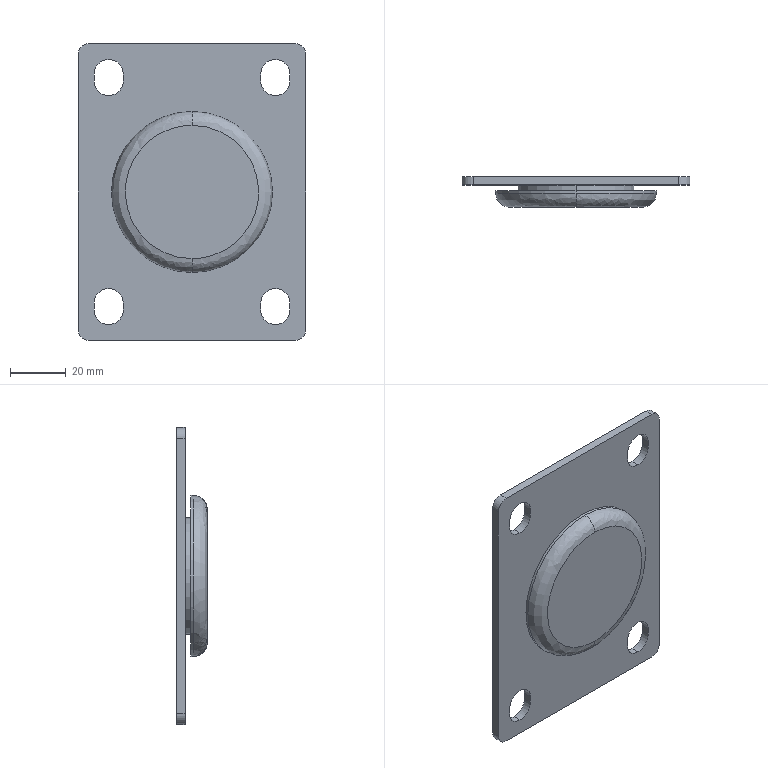Part | SolidWorks | features BaseBody 1 | 1 solid | 47 faces | box 82 x 11 x 107 mm | volume 39892 mm3 | cylinder 26 | plane 19 | spline 2 | commonest cylinder face diameters 10.5 x12 8 x4 25 x2 40 x2 42 x2 58 x2
STEP:
#1=CARTESIAN_POINT('',(0.,55.5,-57.3));
#2=VERTEX_POINT('',#1);
#3=CARTESIAN_POINT('',(0.,55.5,0.7));
#4=VERTEX_POINT('',#3);
#5=CARTESIAN_POINT('',(0.,55.5,-28.3));
#6=DIRECTION('',(0.,1.,0.));
#7=DIRECTION('',(0.,0.,-1.));
#8=AXIS2_PLACEMENT_3D('',#5,#6,#7);
#9=CIRCLE('',#8,29.);
#10=EDGE_CURVE('',#2,#4,#9,.T.);
#11=ORIENTED_EDGE('',*,*,#10,.F.);
#12=CARTESIAN_POINT('',(0.,50.5,-52.3));
#13=VERTEX_POINT('',#12);
#14=CARTESIAN_POINT('',(0.,55.5,-52.3));
#15=DIRECTION('',(-1.,0.,0.));
#16=DIRECTION('',(0.,0.,-1.));
#17=AXIS2_PLACEMENT_3D('',#14,#15,#16);
#18=CIRCLE('',#17,5.);
#19=EDGE_CURVE('',#2,#13,#18,.T.);
#20=ORIENTED_EDGE('',*,*,#19,.T.);
#21=CARTESIAN_POINT('',(0.,50.5,-4.3));
#22=VERTEX_POINT('',#21);
#23=CARTESIAN_POINT('',(0.,50.5,-52.3));
#24=CARTESIAN_POINT('',(-48.,50.5,-52.3));
#25=CARTESIAN_POINT('',(-48.,50.5,-4.3));
#26=CARTESIAN_POINT('',(0.,50.5,-4.3));
#27=(BOUNDED_CURVE()B_SPLINE_CURVE(3,(#23,#24,#25,#26),.UNSPECIFIED.,.F.,.F.)B_SPLINE_CURVE_WITH_KNOTS((4,4),(0.5,1.),.UNSPECIFIED.)CURVE()GEOMETRIC_REPRESENTATION_ITEM()RATIONAL_B_SPLINE_CURVE((1.,0.3333,0.3333,1.))REPRESENTATION_ITEM(''));
#28=EDGE_CURVE('',#13,#22,#27,.T.);
#29=ORIENTED_EDGE('',*,*,#28,.T.);
#30=CARTESIAN_POINT('',(0.,55.5,-4.3));
#31=DIRECTION('',(1.,0.,0.));
#32=DIRECTION('',(0.,0.,1.));
#33=AXIS2_PLACEMENT_3D('',#30,#31,#32);
#34=CIRCLE('',#33,5.);
#35=EDGE_CURVE('',#4,#22,#34,.T.);
#36=ORIENTED_EDGE('',*,*,#35,.F.);
#37=EDGE_LOOP('',(#11,#20,#29,#36));
#38=FACE_OUTER_BOUND('',#37,.T.);
#39=CARTESIAN_POINT('',(0.,55.5,-57.3));
#40=CARTESIAN_POINT('',(-58.,55.5,-57.3));
#41=CARTESIAN_POINT('',(-58.,55.5,0.7));
#42=CARTESIAN_POINT('',(0.,55.5,0.7));
#43=CARTESIAN_POINT('',(0.,52.571,-57.3));
#44=CARTESIAN_POINT('',(-58.,52.571,-57.3));
#45=CARTESIAN_POINT('',(-58.,52.571,0.7));
#46=CARTESIAN_POINT('',(0.,52.571,0.7));
#47=CARTESIAN_POINT('',(0.,50.5,-55.229));
#48=CARTESIAN_POINT('',(-53.858,50.5,-55.229));
#49=CARTESIAN_POINT('',(-53.858,50.5,-1.371));
#50=CARTESIAN_POINT('',(0.,50.5,-1.371));
#51=CARTESIAN_POINT('',(0.,50.5,-52.3));
#52=CARTESIAN_POINT('',(-48.,50.5,-52.3));
#53=CARTESIAN_POINT('',(-48.,50.5,-4.3));
#54=CARTESIAN_POINT('',(0.,50.5,-4.3));
#55=(BOUNDED_SURFACE()B_SPLINE_SURFACE(3,3,((#39,#40,#41,#42),(#43,#44,#45,#46),(#47,#48,#49,#50),(#51,#52,#53,#54)),.UNSPECIFIED.,.F.,.F.,.F.)B_SPLINE_SURFACE_WITH_KNOTS((4,4),(4,4),(0.,1.),(0.,1.),.UNSPECIFIED.)GEOMETRIC_REPRESENTATION_ITEM()RATIONAL_B_SPLINE_SURFACE(((1.,0.3333,0.3333,1.),(0.8047,0.2682,0.2682,0.8047),(0.8047,0.2682,0.2682,0.8047),(1.,0.3333,0.3333,1.)))REPRESENTATION_ITEM('')SURFACE());
#56=ADVANCED_FACE('',(#38),#55,.T.);
#57=CARTESIAN_POINT('',(30.,61.5,6.45));
#58=VERTEX_POINT('',#57);
#59=CARTESIAN_POINT('',(35.25,61.5,11.7));
#60=VERTEX_POINT('',#59);
#61=CARTESIAN_POINT('',(30.,61.5,11.7));
#62=DIRECTION('',(0.,-1.,0.));
#63=DIRECTION('',(0.,0.,-1.));
#64=AXIS2_PLACEMENT_3D('',#61,#62,#63);
#65=CIRCLE('',#64,5.25);
#66=EDGE_CURVE('',#58,#60,#65,.T.);
#67=ORIENTED_EDGE('',*,*,#66,.F.);
#68=CARTESIAN_POINT('',(30.,58.5,6.45));
#69=VERTEX_POINT('',#68);
#70=CARTESIAN_POINT('',(30.,58.5,6.45));
#71=DIRECTION('',(0.,-1.,0.));
#72=VECTOR('',#71,1000.);
#73=LINE('',#70,#72);
#74=EDGE_CURVE('',#58,#69,#73,.T.);
#75=ORIENTED_EDGE('',*,*,#74,.T.);
#76=CARTESIAN_POINT('',(35.25,58.5,11.7));
#77=VERTEX_POINT('',#76);
#78=CARTESIAN_POINT('',(30.,58.5,11.7));
#79=DIRECTION('',(0.,-1.,0.));
#80=DIRECTION('',(0.,0.,-1.));
#81=AXIS2_PLACEMENT_3D('',#78,#79,#80);
#82=CIRCLE('',#81,5.25);
#83=EDGE_CURVE('',#69,#77,#82,.T.);
#84=ORIENTED_EDGE('',*,*,#83,.T.);
#85=CARTESIAN_POINT('',(35.25,58.5,11.7));
#86=DIRECTION('',(0.,-1.,0.));
#87=VECTOR('',#86,1000.);
#88=LINE('',#85,#87);
#89=EDGE_CURVE('',#60,#77,#88,.T.);
#90=ORIENTED_EDGE('',*,*,#89,.F.);
#91=EDGE_LOOP('',(#67,#75,#84,#90));
#92=FACE_OUTER_BOUND('',#91,.T.);
#93=CARTESIAN_POINT('',(30.,58.5,11.7));
#94=DIRECTION('',(0.,-1.,0.));
#95=DIRECTION('',(0.,0.,-1.));
#96=AXIS2_PLACEMENT_3D('',#93,#94,#95);
#97=CYLINDRICAL_SURFACE('',#96,5.25);
#98=ADVANCED_FACE('',(#92),#97,.F.);
#99=CARTESIAN_POINT('',(30.,61.5,-76.05));
#100=VERTEX_POINT('',#99);
#101=CARTESIAN_POINT('',(35.25,61.5,-70.8));
#102=VERTEX_POINT('',#101);
#103=CARTESIAN_POINT('',(30.,61.5,-70.8));
#104=DIRECTION('',(0.,-1.,0.));
#105=DIRECTION('',(0.,0.,-1.));
#106=AXIS2_PLACEMENT_3D('',#103,#104,#105);
#107=CIRCLE('',#106,5.25);
#108=EDGE_CURVE('',#100,#102,#107,.T.);
#109=ORIENTED_EDGE('',*,*,#108,.F.);
#110=CARTESIAN_POINT('',(30.,58.5,-76.05));
#111=VERTEX_POINT('',#110);
#112=CARTESIAN_POINT('',(30.,58.5,-76.05));
#113=DIRECTION('',(0.,-1.,0.));
#114=VECTOR('',#113,1000.);
#115=LINE('',#112,#114);
#116=EDGE_CURVE('',#100,#111,#115,.T.);
#117=ORIENTED_EDGE('',*,*,#116,.T.);
#118=CARTESIAN_POINT('',(35.25,58.5,-70.8));
#119=VERTEX_POINT('',#118);
#120=CARTESIAN_POINT('',(30.,58.5,-70.8));
#121=DIRECTION('',(0.,-1.,0.));
#122=DIRECTION('',(0.,0.,-1.));
#123=AXIS2_PLACEMENT_3D('',#120,#121,#122);
#124=CIRCLE('',#123,5.25);
#125=EDGE_CURVE('',#111,#119,#124,.T.);
#126=ORIENTED_EDGE('',*,*,#125,.T.);
#127=CARTESIAN_POINT('',(35.25,58.5,-70.8));
#128=DIRECTION('',(0.,1.,0.));
#129=VECTOR('',#128,1000.);
#130=LINE('',#127,#129);
#131=EDGE_CURVE('',#119,#102,#130,.T.);
#132=ORIENTED_EDGE('',*,*,#131,.T.);
#133=EDGE_LOOP('',(#109,#117,#126,#132));
#134=FACE_OUTER_BOUND('',#133,.T.);
#135=CARTESIAN_POINT('',(30.,58.5,-70.8));
#136=DIRECTION('',(0.,-1.,0.));
#137=DIRECTION('',(0.,0.,-1.));
#138=AXIS2_PLACEMENT_3D('',#135,#136,#137);
#139=CYLINDRICAL_SURFACE('',#138,5.25);
#140=ADVANCED_FACE('',(#134),#139,.F.);
#141=CARTESIAN_POINT('',(-30.,61.5,6.45));
#142=VERTEX_POINT('',#141);
#143=CARTESIAN_POINT('',(-24.75,61.5,11.7));
#144=VERTEX_POINT('',#143);
#145=CARTESIAN_POINT('',(-30.,61.5,11.7));
#146=DIRECTION('',(0.,-1.,0.));
#147=DIRECTION('',(0.,0.,-1.));
#148=AXIS2_PLACEMENT_3D('',#145,#146,#147);
#149=CIRCLE('',#148,5.25);
#150=EDGE_CURVE('',#142,#144,#149,.T.);
#151=ORIENTED_EDGE('',*,*,#150,.F.);
#152=CARTESIAN_POINT('',(-30.,58.5,6.45));
#153=VERTEX_POINT('',#152);
#154=CARTESIAN_POINT('',(-30.,58.5,6.45));
#155=DIRECTION('',(0.,-1.,0.));
#156=VECTOR('',#155,1000.);
#157=LINE('',#154,#156);
#158=EDGE_CURVE('',#142,#153,#157,.T.);
#159=ORIENTED_EDGE('',*,*,#158,.T.);
#160=CARTESIAN_POINT('',(-24.75,58.5,11.7));
#161=VERTEX_POINT('',#160);
#162=CARTESIAN_POINT('',(-30.,58.5,11.7));
#163=DIRECTION('',(0.,-1.,0.));
#164=DIRECTION('',(0.,0.,-1.));
#165=AXIS2_PLACEMENT_3D('',#162,#163,#164);
#166=CIRCLE('',#165,5.25);
#167=EDGE_CURVE('',#153,#161,#166,.T.);
#168=ORIENTED_EDGE('',*,*,#167,.T.);
#169=CARTESIAN_POINT('',(-24.75,58.5,11.7));
#170=DIRECTION('',(0.,-1.,0.));
#171=VECTOR('',#170,1000.);
#172=LINE('',#169,#171);
#173=EDGE_CURVE('',#144,#161,#172,.T.);
#174=ORIENTED_EDGE('',*,*,#173,.F.);
#175=EDGE_LOOP('',(#151,#159,#168,#174));
#176=FACE_OUTER_BOUND('',#175,.T.);
#177=CARTESIAN_POINT('',(-30.,58.5,11.7));
#178=DIRECTION('',(0.,-1.,0.));
#179=DIRECTION('',(0.,0.,-1.));
#180=AXIS2_PLACEMENT_3D('',#177,#178,#179);
#181=CYLINDRICAL_SURFACE('',#180,5.25);
#182=ADVANCED_FACE('',(#176),#181,.F.);
#183=CARTESIAN_POINT('',(-30.,61.5,-76.05));
#184=VERTEX_POINT('',#183);
#185=CARTESIAN_POINT('',(-24.75,61.5,-70.8));
#186=VERTEX_POINT('',#185);
#187=CARTESIAN_POINT('',(-30.,61.5,-70.8));
#188=DIRECTION('',(0.,-1.,0.));
#189=DIRECTION('',(0.,0.,-1.));
#190=AXIS2_PLACEMENT_3D('',#187,#188,#189);
#191=CIRCLE('',#190,5.25);
#192=EDGE_CURVE('',#184,#186,#191,.T.);
#193=ORIENTED_EDGE('',*,*,#192,.F.);
#194=CARTESIAN_POINT('',(-30.,58.5,-76.05));
#195=VERTEX_POINT('',#194);
#196=CARTESIAN_POINT('',(-30.,58.5,-76.05));
#197=DIRECTION('',(0.,-1.,0.));
#198=VECTOR('',#197,1000.);
#199=LINE('',#196,#198);
#200=EDGE_CURVE('',#184,#195,#199,.T.);
#201=ORIENTED_EDGE('',*,*,#200,.T.);
#202=CARTESIAN_POINT('',(-24.75,58.5,-70.8));
#203=VERTEX_POINT('',#202);
#204=CARTESIAN_POINT('',(-30.,58.5,-70.8));
#205=DIRECTION('',(0.,-1.,0.));
#206=DIRECTION('',(0.,0.,-1.));
#207=AXIS2_PLACEMENT_3D('',#204,#205,#206);
#208=CIRCLE('',#207,5.25);
#209=EDGE_CURVE('',#195,#203,#208,.T.);
#210=ORIENTED_EDGE('',*,*,#209,.T.);
#211=CARTESIAN_POINT('',(-24.75,58.5,-70.8));
#212=DIRECTION('',(0.,1.,0.));
#213=VECTOR('',#212,1000.);
#214=LINE('',#211,#213);
#215=EDGE_CURVE('',#203,#186,#214,.T.);
#216=ORIENTED_EDGE('',*,*,#215,.T.);
#217=EDGE_LOOP('',(#193,#201,#210,#216));
#218=FACE_OUTER_BOUND('',#217,.T.);
#219=CARTESIAN_POINT('',(-30.,58.5,-70.8));
#220=DIRECTION('',(0.,-1.,0.));
#221=DIRECTION('',(0.,0.,-1.));
#222=AXIS2_PLACEMENT_3D('',#219,#220,#221);
#223=CYLINDRICAL_SURFACE('',#222,5.25);
#224=ADVANCED_FACE('',(#218),#223,.F.);
#225=CARTESIAN_POINT('',(0.,58.5,-49.3));
#226=VERTEX_POINT('',#225);
#227=CARTESIAN_POINT('',(0.,58.5,-7.3));
#228=VERTEX_POINT('',#227);
#229=CARTESIAN_POINT('',(0.,58.5,-28.3));
#230=DIRECTION('',(0.,-1.,0.));
#231=DIRECTION('',(0.,0.,-1.));
#232=AXIS2_PLACEMENT_3D('',#229,#230,#231);
#233=CIRCLE('',#232,21.);
#234=EDGE_CURVE('',#226,#228,#233,.T.);
#235=ORIENTED_EDGE('',*,*,#234,.T.);
#236=CARTESIAN_POINT('',(0.,56.5,-7.3));
#237=VERTEX_POINT('',#236);
#238=CARTESIAN_POINT('',(0.,56.5,-7.3));
#239=DIRECTION('',(0.,-1.,0.));
#240=VECTOR('',#239,1000.);
#241=LINE('',#238,#240);
#242=EDGE_CURVE('',#228,#237,#241,.T.);
#243=ORIENTED_EDGE('',*,*,#242,.T.);
#244=CARTESIAN_POINT('',(0.,56.5,-49.3));
#245=VERTEX_POINT('',#244);
#246=CARTESIAN_POINT('',(0.,56.5,-28.3));
#247=DIRECTION('',(0.,1.,0.));
#248=DIRECTION('',(0.,0.,-1.));
#249=AXIS2_PLACEMENT_3D('',#246,#247,#248);
#250=CIRCLE('',#249,21.);
#251=EDGE_CURVE('',#237,#245,#250,.T.);
#252=ORIENTED_EDGE('',*,*,#251,.T.);
#253=CARTESIAN_POINT('',(0.,56.5,-49.3));
#254=DIRECTION('',(0.,-1.,0.));
#255=VECTOR('',#254,1000.);
#256=LINE('',#253,#255);
#257=EDGE_CURVE('',#226,#245,#256,.T.);
#258=ORIENTED_EDGE('',*,*,#257,.F.);
#259=EDGE_LOOP('',(#235,#243,#252,#258));
#260=FACE_OUTER_BOUND('',#259,.T.);
#261=CARTESIAN_POINT('',(0.,56.5,-28.3));
#262=DIRECTION('',(0.,-1.,0.));
#263=DIRECTION('',(0.,0.,-1.));
#264=AXIS2_PLACEMENT_3D('',#261,#262,#263);
#265=CYLINDRICAL_SURFACE('',#264,21.);
#266=ADVANCED_FACE('',(#260),#265,.T.);
#267=CARTESIAN_POINT('',(0.,61.5,1.7));
#268=VERTEX_POINT('',#267);
#269=CARTESIAN_POINT('',(0.,61.5,-58.3));
#270=VERTEX_POINT('',#269);
#271=CARTESIAN_POINT('',(0.,61.5,-28.3));
#272=DIRECTION('',(0.,-1.,0.));
#273=DIRECTION('',(0.,0.,-1.));
#274=AXIS2_PLACEMENT_3D('',#271,#272,#273);
#275=CIRCLE('',#274,30.);
#276=EDGE_CURVE('',#268,#270,#275,.T.);
#277=ORIENTED_EDGE('',*,*,#276,.F.);
#278=CARTESIAN_POINT('',(0.,60.5,1.7));
#279=VERTEX_POINT('',#278);
#280=CARTESIAN_POINT('',(0.,60.5,1.7));
#281=DIRECTION('',(0.,-1.,0.));
#282=VECTOR('',#281,1000.);
#283=LINE('',#280,#282);
#284=EDGE_CURVE('',#268,#279,#283,.T.);
#285=ORIENTED_EDGE('',*,*,#284,.T.);
#286=CARTESIAN_POINT('',(0.,60.5,-58.3));
#287=VERTEX_POINT('',#286);
#288=CARTESIAN_POINT('',(0.,60.5,-28.3));
#289=DIRECTION('',(0.,1.,0.));
#290=DIRECTION('',(0.,0.,-1.));
#291=AXIS2_PLACEMENT_3D('',#288,#289,#290);
#292=CIRCLE('',#291,30.);
#293=EDGE_CURVE('',#287,#279,#292,.T.);
#294=ORIENTED_EDGE('',*,*,#293,.F.);
#295=CARTESIAN_POINT('',(0.,60.5,-58.3));
#296=DIRECTION('',(0.,-1.,0.));
#297=VECTOR('',#296,1000.);
#298=LINE('',#295,#297);
#299=EDGE_CURVE('',#270,#287,#298,.T.);
#300=ORIENTED_EDGE('',*,*,#299,.F.);
#301=EDGE_LOOP('',(#277,#285,#294,#300));
#302=FACE_OUTER_BOUND('',#301,.T.);
#303=CARTESIAN_POINT('',(0.,60.5,-28.3));
#304=DIRECTION('',(0.,-1.,0.));
#305=DIRECTION('',(0.,0.,-1.));
#306=AXIS2_PLACEMENT_3D('',#303,#304,#305);
#307=CYLINDRICAL_SURFACE('',#306,30.);
#308=ADVANCED_FACE('',(#302),#307,.F.);
#309=CARTESIAN_POINT('',(0.,56.5,-57.3));
#310=VERTEX_POINT('',#309);
#311=CARTESIAN_POINT('',(0.,56.5,0.7));
#312=VERTEX_POINT('',#311);
#313=CARTESIAN_POINT('',(0.,56.5,-28.3));
#314=DIRECTION('',(0.,-1.,0.));
#315=DIRECTION('',(0.,0.,-1.));
#316=AXIS2_PLACEMENT_3D('',#313,#314,#315);
#317=CIRCLE('',#316,29.);
#318=EDGE_CURVE('',#310,#312,#317,.T.);
#319=ORIENTED_EDGE('',*,*,#318,.T.);
#320=CARTESIAN_POINT('',(0.,56.5,0.7));
#321=DIRECTION('',(0.,-1.,0.));
#322=VECTOR('',#321,1000.);
#323=LINE('',#320,#322);
#324=EDGE_CURVE('',#312,#4,#323,.T.);
#325=ORIENTED_EDGE('',*,*,#324,.T.);
#326=CARTESIAN_POINT('',(0.,55.5,-28.3));
#327=DIRECTION('',(0.,1.,0.));
#328=DIRECTION('',(0.,0.,-1.));
#329=AXIS2_PLACEMENT_3D('',#326,#327,#328);
#330=CIRCLE('',#329,29.);
#331=EDGE_CURVE('',#4,#2,#330,.T.);
#332=ORIENTED_EDGE('',*,*,#331,.T.);
#333=CARTESIAN_POINT('',(0.,56.5,-57.3));
#334=DIRECTION('',(0.,-1.,0.));
#335=VECTOR('',#334,1000.);
#336=LINE('',#333,#335);
#337=EDGE_CURVE('',#310,#2,#336,.T.);
#338=ORIENTED_EDGE('',*,*,#337,.F.);
#339=EDGE_LOOP('',(#319,#325,#332,#338));
#340=FACE_OUTER_BOUND('',#339,.T.);
#341=CARTESIAN_POINT('',(0.,56.5,-28.3));
#342=DIRECTION('',(0.,-1.,0.));
#343=DIRECTION('',(0.,0.,-1.));
#344=AXIS2_PLACEMENT_3D('',#341,#342,#343);
#345=CYLINDRICAL_SURFACE('',#344,29.);
#346=ADVANCED_FACE('',(#340),#345,.T.);
#347=CARTESIAN_POINT('',(0.,60.5,-8.3));
#348=VERTEX_POINT('',#347);
#349=CARTESIAN_POINT('',(0.,60.5,-48.3));
#350=VERTEX_POINT('',#349);
#351=CARTESIAN_POINT('',(0.,60.5,-28.3));
#352=DIRECTION('',(0.,-1.,0.));
#353=DIRECTION('',(0.,0.,-1.));
#354=AXIS2_PLACEMENT_3D('',#351,#352,#353);
#355=CIRCLE('',#354,20.);
#356=EDGE_CURVE('',#348,#350,#355,.T.);
#357=ORIENTED_EDGE('',*,*,#356,.F.);
#358=CARTESIAN_POINT('',(0.,60.,-8.3));
#359=VERTEX_POINT('',#358);
#360=CARTESIAN_POINT('',(0.,60.,-8.3));
#361=DIRECTION('',(0.,-1.,0.));
#362=VECTOR('',#361,1000.);
#363=LINE('',#360,#362);
#364=EDGE_CURVE('',#348,#359,#363,.T.);
#365=ORIENTED_EDGE('',*,*,#364,.T.);
#366=CARTESIAN_POINT('',(0.,60.,-48.3));
#367=VERTEX_POINT('',#366);
#368=CARTESIAN_POINT('',(0.,60.,-28.3));
#369=DIRECTION('',(0.,1.,0.));
#370=DIRECTION('',(0.,0.,-1.));
#371=AXIS2_PLACEMENT_3D('',#368,#369,#370);
#372=CIRCLE('',#371,20.);
#373=EDGE_CURVE('',#367,#359,#372,.T.);
#374=ORIENTED_EDGE('',*,*,#373,.F.);
#375=CARTESIAN_POINT('',(0.,60.,-48.3));
#376=DIRECTION('',(0.,-1.,0.));
#377=VECTOR('',#376,1000.);
#378=LINE('',#375,#377);
#379=EDGE_CURVE('',#350,#367,#378,.T.);
#380=ORIENTED_EDGE('',*,*,#379,.F.);
#381=EDGE_LOOP('',(#357,#365,#374,#380));
#382=FACE_OUTER_BOUND('',#381,.T.);
#383=CARTESIAN_POINT('',(0.,60.,-28.3));
#384=DIRECTION('',(0.,-1.,0.));
#385=DIRECTION('',(0.,0.,-1.));
#386=AXIS2_PLACEMENT_3D('',#383,#384,#385);
#387=CYLINDRICAL_SURFACE('',#386,20.);
#388=ADVANCED_FACE('',(#382),#387,.F.);
#389=CARTESIAN_POINT('',(0.,61.5,-40.8));
#390=VERTEX_POINT('',#389);
#391=CARTESIAN_POINT('',(0.,61.5,-15.8));
#392=VERTEX_POINT('',#391);
#393=CARTESIAN_POINT('',(0.,61.5,-28.3));
#394=DIRECTION('',(0.,-1.,0.));
#395=DIRECTION('',(0.,0.,-1.));
#396=AXIS2_PLACEMENT_3D('',#393,#394,#395);
#397=CIRCLE('',#396,12.5);
#398=EDGE_CURVE('',#390,#392,#397,.T.);
#399=ORIENTED_EDGE('',*,*,#398,.T.);
#400=CARTESIAN_POINT('',(0.,60.,-15.8));
#401=VERTEX_POINT('',#400);
#402=CARTESIAN_POINT('',(0.,59.,-15.8));
#403=DIRECTION('',(0.,-1.,0.));
#404=VECTOR('',#403,1000.);
#405=LINE('',#402,#404);
#406=EDGE_CURVE('',#392,#401,#405,.T.);
#407=ORIENTED_EDGE('',*,*,#406,.T.);
#408=CARTESIAN_POINT('',(0.,60.,-40.8));
#409=VERTEX_POINT('',#408);
#410=CARTESIAN_POINT('',(0.,60.,-28.3));
#411=DIRECTION('',(0.,-1.,0.));
#412=DIRECTION('',(0.,0.,-1.));
#413=AXIS2_PLACEMENT_3D('',#410,#411,#412);
#414=CIRCLE('',#413,12.5);
#415=EDGE_CURVE('',#409,#401,#414,.T.);
#416=ORIENTED_EDGE('',*,*,#415,.F.);
#417=CARTESIAN_POINT('',(0.,59.,-40.8));
#418=DIRECTION('',(0.,-1.,0.));
#419=VECTOR('',#418,1000.);
#420=LINE('',#417,#419);
#421=EDGE_CURVE('',#390,#409,#420,.T.);
#422=ORIENTED_EDGE('',*,*,#421,.F.);
#423=EDGE_LOOP('',(#399,#407,#416,#422));
#424=FACE_OUTER_BOUND('',#423,.T.);
#425=CARTESIAN_POINT('',(0.,59.,-28.3));
#426=DIRECTION('',(0.,-1.,0.));
#427=DIRECTION('',(0.,0.,-1.));
#428=AXIS2_PLACEMENT_3D('',#425,#426,#427);
#429=CYLINDRICAL_SURFACE('',#428,12.5);
#430=ADVANCED_FACE('',(#424),#429,.T.);
#431=CARTESIAN_POINT('',(37.,58.5,-81.8));
#432=VERTEX_POINT('',#431);
#433=CARTESIAN_POINT('',(-37.,58.5,-81.8));
#434=VERTEX_POINT('',#433);
#435=CARTESIAN_POINT('',(-37.,58.5,-81.8));
#436=DIRECTION('',(-1.,0.,0.));
#437=VECTOR('',#436,1000.);
#438=LINE('',#435,#437);
#439=EDGE_CURVE('',#432,#434,#438,.T.);
#440=ORIENTED_EDGE('',*,*,#439,.F.);
#441=CARTESIAN_POINT('',(41.,58.5,-77.8));
#442=VERTEX_POINT('',#441);
#443=CARTESIAN_POINT('',(37.,58.5,-77.8));
#444=DIRECTION('',(0.,1.,0.));
#445=DIRECTION('',(0.,0.,-1.));
#446=AXIS2_PLACEMENT_3D('',#443,#444,#445);
#447=CIRCLE('',#446,4.);
#448=EDGE_CURVE('',#442,#432,#447,.T.);
#449=ORIENTED_EDGE('',*,*,#448,.F.);
#450=CARTESIAN_POINT('',(41.,58.5,21.2));
#451=VERTEX_POINT('',#450);
#452=CARTESIAN_POINT('',(41.,58.5,-77.8));
#453=DIRECTION('',(0.,0.,-1.));
#454=VECTOR('',#453,1000.);
#455=LINE('',#452,#454);
#456=EDGE_CURVE('',#451,#442,#455,.T.);
#457=ORIENTED_EDGE('',*,*,#456,.F.);
#458=CARTESIAN_POINT('',(37.,58.5,25.2));
#459=VERTEX_POINT('',#458);
#460=CARTESIAN_POINT('',(37.,58.5,21.2));
#461=DIRECTION('',(0.,1.,0.));
#462=DIRECTION('',(0.,0.,-1.));
#463=AXIS2_PLACEMENT_3D('',#460,#461,#462);
#464=CIRCLE('',#463,4.);
#465=EDGE_CURVE('',#459,#451,#464,.T.);
#466=ORIENTED_EDGE('',*,*,#465,.F.);
#467=CARTESIAN_POINT('',(-37.,58.5,25.2));
#468=VERTEX_POINT('',#467);
#469=CARTESIAN_POINT('',(-37.,58.5,25.2));
#470=DIRECTION('',(1.,0.,0.));
#471=VECTOR('',#470,1000.);
#472=LINE('',#469,#471);
#473=EDGE_CURVE('',#468,#459,#472,.T.);
#474=ORIENTED_EDGE('',*,*,#473,.F.);
#475=CARTESIAN_POINT('',(-41.,58.5,21.2));
#476=VERTEX_POINT('',#475);
#477=CARTESIAN_POINT('',(-37.,58.5,21.2));
#478=DIRECTION('',(0.,1.,0.));
#479=DIRECTION('',(0.,0.,-1.));
#480=AXIS2_PLACEMENT_3D('',#477,#478,#479);
#481=CIRCLE('',#480,4.);
#482=EDGE_CURVE('',#476,#468,#481,.T.);
#483=ORIENTED_EDGE('',*,*,#482,.F.);
#484=CARTESIAN_POINT('',(-41.,58.5,-77.8));
#485=VERTEX_POINT('',#484);
#486=CARTESIAN_POINT('',(-41.,58.5,-77.8));
#487=DIRECTION('',(0.,0.,1.));
#488=VECTOR('',#487,1000.);
#489=LINE('',#486,#488);
#490=EDGE_CURVE('',#485,#476,#489,.T.);
#491=ORIENTED_EDGE('',*,*,#490,.F.);
#492=CARTESIAN_POINT('',(-37.,58.5,-77.8));
#493=DIRECTION('',(0.,1.,0.));
#494=DIRECTION('',(0.,0.,-1.));
#495=AXIS2_PLACEMENT_3D('',#492,#493,#494);
#496=CIRCLE('',#495,4.);
#497=EDGE_CURVE('',#434,#485,#496,.T.);
#498=ORIENTED_EDGE('',*,*,#497,.F.);
#499=EDGE_LOOP('',(#440,#449,#457,#466,#474,#483,#491,#498));
#500=FACE_OUTER_BOUND('',#499,.T.);
#501=CARTESIAN_POINT('',(24.75,58.5,14.2));
#502=VERTEX_POINT('',#501);
#503=CARTESIAN_POINT('',(24.75,58.5,11.7));
#504=VERTEX_POINT('',#503);
#505=CARTESIAN_POINT('',(24.75,58.5,-77.8));
#506=DIRECTION('',(0.,0.,-1.));
#507=VECTOR('',#506,1000.);
#508=LINE('',#505,#507);
#509=EDGE_CURVE('',#502,#504,#508,.T.);
#510=ORIENTED_EDGE('',*,*,#509,.F.);
#511=CARTESIAN_POINT('',(35.25,58.5,14.2));
#512=VERTEX_POINT('',#511);
#513=CARTESIAN_POINT('',(30.,58.5,14.2));
#514=DIRECTION('',(0.,-1.,0.));
#515=DIRECTION('',(0.,0.,-1.));
#516=AXIS2_PLACEMENT_3D('',#513,#514,#515);
#517=CIRCLE('',#516,5.25);
#518=EDGE_CURVE('',#512,#502,#517,.T.);
#519=ORIENTED_EDGE('',*,*,#518,.F.);
#520=CARTESIAN_POINT('',(35.25,58.5,-77.8));
#521=DIRECTION('',(0.,0.,1.));
#522=VECTOR('',#521,1000.);
#523=LINE('',#520,#522);
#524=EDGE_CURVE('',#77,#512,#523,.T.);
#525=ORIENTED_EDGE('',*,*,#524,.F.);
#526=ORIENTED_EDGE('',*,*,#83,.F.);
#527=CARTESIAN_POINT('',(30.,58.5,11.7));
#528=DIRECTION('',(0.,-1.,0.));
#529=DIRECTION('',(0.,0.,-1.));
#530=AXIS2_PLACEMENT_3D('',#527,#528,#529);
#531=CIRCLE('',#530,5.25);
#532=EDGE_CURVE('',#504,#69,#531,.T.);
#533=ORIENTED_EDGE('',*,*,#532,.F.);
#534=EDGE_LOOP('',(#510,#519,#525,#526,#533));
#535=FACE_BOUND('',#534,.T.);
#536=CARTESIAN_POINT('',(35.25,58.5,-68.3));
#537=VERTEX_POINT('',#536);
#538=CARTESIAN_POINT('',(24.75,58.5,-68.3));
#539=VERTEX_POINT('',#538);
#540=CARTESIAN_POINT('',(30.,58.5,-68.3));
#541=DIRECTION('',(0.,-1.,0.));
#542=DIRECTION('',(0.,0.,-1.));
#543=AXIS2_PLACEMENT_3D('',#540,#541,#542);
#544=CIRCLE('',#543,5.25);
#545=EDGE_CURVE('',#537,#539,#544,.T.);
#546=ORIENTED_EDGE('',*,*,#545,.F.);
#547=CARTESIAN_POINT('',(35.25,58.5,-77.8));
#548=DIRECTION('',(0.,0.,1.));
#549=VECTOR('',#548,1000.);
#550=LINE('',#547,#549);
#551=EDGE_CURVE('',#119,#537,#550,.T.);
#552=ORIENTED_EDGE('',*,*,#551,.F.);
#553=ORIENTED_EDGE('',*,*,#125,.F.);
#554=CARTESIAN_POINT('',(24.75,58.5,-70.8));
#555=VERTEX_POINT('',#554);
#556=CARTESIAN_POINT('',(30.,58.5,-70.8));
#557=DIRECTION('',(0.,-1.,0.));
#558=DIRECTION('',(0.,0.,-1.));
#559=AXIS2_PLACEMENT_3D('',#556,#557,#558);
#560=CIRCLE('',#559,5.25);
#561=EDGE_CURVE('',#555,#111,#560,.T.);
#562=ORIENTED_EDGE('',*,*,#561,.F.);
#563=CARTESIAN_POINT('',(24.75,58.5,-77.8));
#564=DIRECTION('',(0.,0.,-1.));
#565=VECTOR('',#564,1000.);
#566=LINE('',#563,#565);
#567=EDGE_CURVE('',#539,#555,#566,.T.);
#568=ORIENTED_EDGE('',*,*,#567,.F.);
#569=EDGE_LOOP('',(#546,#552,#553,#562,#568));
#570=FACE_BOUND('',#569,.T.);
#571=CARTESIAN_POINT('',(-35.25,58.5,14.2));
#572=VERTEX_POINT('',#571);
#573=CARTESIAN_POINT('',(-35.25,58.5,11.7));
#574=VERTEX_POINT('',#573);
#575=CARTESIAN_POINT('',(-35.25,58.5,-77.8));
#576=DIRECTION('',(0.,0.,-1.));
#577=VECTOR('',#576,1000.);
#578=LINE('',#575,#577);
#579=EDGE_CURVE('',#572,#574,#578,.T.);
#580=ORIENTED_EDGE('',*,*,#579,.F.);
#581=CARTESIAN_POINT('',(-24.75,58.5,14.2));
#582=VERTEX_POINT('',#581);
#583=CARTESIAN_POINT('',(-30.,58.5,14.2));
#584=DIRECTION('',(0.,-1.,0.));
#585=DIRECTION('',(0.,0.,-1.));
#586=AXIS2_PLACEMENT_3D('',#583,#584,#585);
#587=CIRCLE('',#586,5.25);
#588=EDGE_CURVE('',#582,#572,#587,.T.);
#589=ORIENTED_EDGE('',*,*,#588,.F.);
#590=CARTESIAN_POINT('',(-24.75,58.5,-77.8));
#591=DIRECTION('',(0.,0.,1.));
#592=VECTOR('',#591,1000.);
#593=LINE('',#590,#592);
#594=EDGE_CURVE('',#161,#582,#593,.T.);
#595=ORIENTED_EDGE('',*,*,#594,.F.);
#596=ORIENTED_EDGE('',*,*,#167,.F.);
#597=CARTESIAN_POINT('',(-30.,58.5,11.7));
#598=DIRECTION('',(0.,-1.,0.));
#599=DIRECTION('',(0.,0.,-1.));
#600=AXIS2_PLACEMENT_3D('',#597,#598,#599);
#601=CIRCLE('',#600,5.25);
#602=EDGE_CURVE('',#574,#153,#601,.T.);
#603=ORIENTED_EDGE('',*,*,#602,.F.);
#604=EDGE_LOOP('',(#580,#589,#595,#596,#603));
#605=FACE_BOUND('',#604,.T.);
#606=CARTESIAN_POINT('',(-24.75,58.5,-68.3));
#607=VERTEX_POINT('',#606);
#608=CARTESIAN_POINT('',(-35.25,58.5,-68.3));
#609=VERTEX_POINT('',#608);
#610=CARTESIAN_POINT('',(-30.,58.5,-68.3));
#611=DIRECTION('',(0.,-1.,0.));
#612=DIRECTION('',(0.,0.,-1.));
#613=AXIS2_PLACEMENT_3D('',#610,#611,#612);
#614=CIRCLE('',#613,5.25);
#615=EDGE_CURVE('',#607,#609,#614,.T.);
#616=ORIENTED_EDGE('',*,*,#615,.F.);
#617=CARTESIAN_POINT('',(-24.75,58.5,-77.8));
#618=DIRECTION('',(0.,0.,1.));
#619=VECTOR('',#618,1000.);
#620=LINE('',#617,#619);
#621=EDGE_CURVE('',#203,#607,#620,.T.);
#622=ORIENTED_EDGE('',*,*,#621,.F.);
#623=ORIENTED_EDGE('',*,*,#209,.F.);
#624=CARTESIAN_POINT('',(-35.25,58.5,-70.8));
#625=VERTEX_POINT('',#624);
#626=CARTESIAN_POINT('',(-30.,58.5,-70.8));
#627=DIRECTION('',(0.,-1.,0.));
#628=DIRECTION('',(0.,0.,-1.));
#629=AXIS2_PLACEMENT_3D('',#626,#627,#628);
#630=CIRCLE('',#629,5.25);
#631=EDGE_CURVE('',#625,#195,#630,.T.);
#632=ORIENTED_EDGE('',*,*,#631,.F.);
#633=CARTESIAN_POINT('',(-35.25,58.5,-77.8));
#634=DIRECTION('',(0.,0.,-1.));
#635=VECTOR('',#634,1000.);
#636=LINE('',#633,#635);
#637=EDGE_CURVE('',#609,#625,#636,.T.);
#638=ORIENTED_EDGE('',*,*,#637,.F.);
#639=EDGE_LOOP('',(#616,#622,#623,#632,#638));
#640=FACE_BOUND('',#639,.T.);
#641=ORIENTED_EDGE('',*,*,#234,.F.);
#642=CARTESIAN_POINT('',(0.,58.5,-28.3));
#643=DIRECTION('',(0.,-1.,0.));
#644=DIRECTION('',(0.,0.,-1.));
#645=AXIS2_PLACEMENT_3D('',#642,#643,#644);
#646=CIRCLE('',#645,21.);
#647=EDGE_CURVE('',#228,#226,#646,.T.);
#648=ORIENTED_EDGE('',*,*,#647,.F.);
#649=EDGE_LOOP('',(#641,#648));
#650=FACE_BOUND('',#649,.T.);
#651=CARTESIAN_POINT('',(-37.,58.5,-77.8));
#652=DIRECTION('',(0.,1.,0.));
#653=DIRECTION('',(0.,0.,1.));
#654=AXIS2_PLACEMENT_3D('',#651,#652,#653);
#655=PLANE('',#654);
#656=ADVANCED_FACE('',(#500,#535,#570,#605,#640,#650),#655,.F.);
#657=ORIENTED_EDGE('',*,*,#497,.T.);
#658=CARTESIAN_POINT('',(-41.,61.5,-77.8));
#659=VERTEX_POINT('',#658);
#660=CARTESIAN_POINT('',(-41.,58.5,-77.8));
#661=DIRECTION('',(0.,1.,0.));
#662=VECTOR('',#661,1000.);
#663=LINE('',#660,#662);
#664=EDGE_CURVE('',#485,#659,#663,.T.);
#665=ORIENTED_EDGE('',*,*,#664,.T.);
#666=CARTESIAN_POINT('',(-37.,61.5,-81.8));
#667=VERTEX_POINT('',#666);
#668=CARTESIAN_POINT('',(-37.,61.5,-77.8));
#669=DIRECTION('',(0.,-1.,0.));
#670=DIRECTION('',(0.,0.,-1.));
#671=AXIS2_PLACEMENT_3D('',#668,#669,#670);
#672=CIRCLE('',#671,4.);
#673=EDGE_CURVE('',#659,#667,#672,.T.);
#674=ORIENTED_EDGE('',*,*,#673,.T.);
#675=CARTESIAN_POINT('',(-37.,58.5,-81.8));
#676=DIRECTION('',(0.,-1.,0.));
#677=VECTOR('',#676,1000.);
#678=LINE('',#675,#677);
#679=EDGE_CURVE('',#667,#434,#678,.T.);
#680=ORIENTED_EDGE('',*,*,#679,.T.);
#681=EDGE_LOOP('',(#657,#665,#674,#680));
#682=FACE_OUTER_BOUND('',#681,.T.);
#683=CARTESIAN_POINT('',(-37.,58.5,-77.8));
#684=DIRECTION('',(0.,-1.,0.));
#685=DIRECTION('',(0.,0.,-1.));
#686=AXIS2_PLACEMENT_3D('',#683,#684,#685);
#687=CYLINDRICAL_SURFACE('',#686,4.);
#688=ADVANCED_FACE('',(#682),#687,.T.);
#689=ORIENTED_EDGE('',*,*,#439,.T.);
#690=ORIENTED_EDGE('',*,*,#679,.F.);
#691=CARTESIAN_POINT('',(37.,61.5,-81.8));
#692=VERTEX_POINT('',#691);
#693=CARTESIAN_POINT('',(37.,61.5,-81.8));
#694=DIRECTION('',(1.,0.,0.));
#695=VECTOR('',#694,1000.);
#696=LINE('',#693,#695);
#697=EDGE_CURVE('',#667,#692,#696,.T.);
#698=ORIENTED_EDGE('',*,*,#697,.T.);
#699=CARTESIAN_POINT('',(37.,58.5,-81.8));
#700=DIRECTION('',(0.,-1.,0.));
#701=VECTOR('',#700,1000.);
#702=LINE('',#699,#701);
#703=EDGE_CURVE('',#692,#432,#702,.T.);
#704=ORIENTED_EDGE('',*,*,#703,.T.);
#705=EDGE_LOOP('',(#689,#690,#698,#704));
#706=FACE_OUTER_BOUND('',#705,.T.);
#707=CARTESIAN_POINT('',(37.,58.5,-81.8));
#708=DIRECTION('',(0.,0.,-1.));
#709=DIRECTION('',(-1.,0.,0.));
#710=AXIS2_PLACEMENT_3D('',#707,#708,#709);
#711=PLANE('',#710);
#712=ADVANCED_FACE('',(#706),#711,.T.);
#713=ORIENTED_EDGE('',*,*,#448,.T.);
#714=ORIENTED_EDGE('',*,*,#703,.F.);
#715=CARTESIAN_POINT('',(41.,61.5,-77.8));
#716=VERTEX_POINT('',#715);
#717=CARTESIAN_POINT('',(37.,61.5,-77.8));
#718=DIRECTION('',(0.,-1.,0.));
#719=DIRECTION('',(0.,0.,-1.));
#720=AXIS2_PLACEMENT_3D('',#717,#718,#719);
#721=CIRCLE('',#720,4.);
#722=EDGE_CURVE('',#692,#716,#721,.T.);
#723=ORIENTED_EDGE('',*,*,#722,.T.);
#724=CARTESIAN_POINT('',(41.,58.5,-77.8));
#725=DIRECTION('',(0.,-1.,0.));
#726=VECTOR('',#725,1000.);
#727=LINE('',#724,#726);
#728=EDGE_CURVE('',#716,#442,#727,.T.);
#729=ORIENTED_EDGE('',*,*,#728,.T.);
#730=EDGE_LOOP('',(#713,#714,#723,#729));
#731=FACE_OUTER_BOUND('',#730,.T.);
#732=CARTESIAN_POINT('',(37.,58.5,-77.8));
#733=DIRECTION('',(0.,-1.,0.));
#734=DIRECTION('',(0.,0.,-1.));
#735=AXIS2_PLACEMENT_3D('',#732,#733,#734);
#736=CYLINDRICAL_SURFACE('',#735,4.);
#737=ADVANCED_FACE('',(#731),#736,.T.);
#738=ORIENTED_EDGE('',*,*,#456,.T.);
#739=ORIENTED_EDGE('',*,*,#728,.F.);
#740=CARTESIAN_POINT('',(41.,61.5,21.2));
#741=VERTEX_POINT('',#740);
#742=CARTESIAN_POINT('',(41.,61.5,21.2));
#743=DIRECTION('',(0.,0.,1.));
#744=VECTOR('',#743,1000.);
#745=LINE('',#742,#744);
#746=EDGE_CURVE('',#716,#741,#745,.T.);
#747=ORIENTED_EDGE('',*,*,#746,.T.);
#748=CARTESIAN_POINT('',(41.,58.5,21.2));
#749=DIRECTION('',(0.,-1.,0.));
#750=VECTOR('',#749,1000.);
#751=LINE('',#748,#750);
#752=EDGE_CURVE('',#741,#451,#751,.T.);
#753=ORIENTED_EDGE('',*,*,#752,.T.);
#754=EDGE_LOOP('',(#738,#739,#747,#753));
#755=FACE_OUTER_BOUND('',#754,.T.);
#756=CARTESIAN_POINT('',(41.,58.5,21.2));
#757=DIRECTION('',(1.,0.,0.));
#758=DIRECTION('',(0.,0.,-1.));
#759=AXIS2_PLACEMENT_3D('',#756,#757,#758);
#760=PLANE('',#759);
#761=ADVANCED_FACE('',(#755),#760,.T.);
#762=ORIENTED_EDGE('',*,*,#465,.T.);
#763=ORIENTED_EDGE('',*,*,#752,.F.);
#764=CARTESIAN_POINT('',(37.,61.5,25.2));
#765=VERTEX_POINT('',#764);
#766=CARTESIAN_POINT('',(37.,61.5,21.2));
#767=DIRECTION('',(0.,-1.,0.));
#768=DIRECTION('',(0.,0.,-1.));
#769=AXIS2_PLACEMENT_3D('',#766,#767,#768);
#770=CIRCLE('',#769,4.);
#771=EDGE_CURVE('',#741,#765,#770,.T.);
#772=ORIENTED_EDGE('',*,*,#771,.T.);
#773=CARTESIAN_POINT('',(37.,58.5,25.2));
#774=DIRECTION('',(0.,-1.,0.));
#775=VECTOR('',#774,1000.);
#776=LINE('',#773,#775);
#777=EDGE_CURVE('',#765,#459,#776,.T.);
#778=ORIENTED_EDGE('',*,*,#777,.T.);
#779=EDGE_LOOP('',(#762,#763,#772,#778));
#780=FACE_OUTER_BOUND('',#779,.T.);
#781=CARTESIAN_POINT('',(37.,58.5,21.2));
#782=DIRECTION('',(0.,-1.,0.));
#783=DIRECTION('',(0.,0.,-1.));
#784=AXIS2_PLACEMENT_3D('',#781,#782,#783);
#785=CYLINDRICAL_SURFACE('',#784,4.);
#786=ADVANCED_FACE('',(#780),#785,.T.);
#787=ORIENTED_EDGE('',*,*,#473,.T.);
#788=ORIENTED_EDGE('',*,*,#777,.F.);
#789=CARTESIAN_POINT('',(-37.,61.5,25.2));
#790=VERTEX_POINT('',#789);
#791=CARTESIAN_POINT('',(-37.,61.5,25.2));
#792=DIRECTION('',(-1.,0.,0.));
#793=VECTOR('',#792,1000.);
#794=LINE('',#791,#793);
#795=EDGE_CURVE('',#765,#790,#794,.T.);
#796=ORIENTED_EDGE('',*,*,#795,.T.);
#797=CARTESIAN_POINT('',(-37.,58.5,25.2));
#798=DIRECTION('',(0.,-1.,0.));
#799=VECTOR('',#798,1000.);
#800=LINE('',#797,#799);
#801=EDGE_CURVE('',#790,#468,#800,.T.);
#802=ORIENTED_EDGE('',*,*,#801,.T.);
#803=EDGE_LOOP('',(#787,#788,#796,#802));
#804=FACE_OUTER_BOUND('',#803,.T.);
#805=CARTESIAN_POINT('',(-37.,58.5,25.2));
#806=DIRECTION('',(0.,0.,1.));
#807=DIRECTION('',(1.,0.,0.));
#808=AXIS2_PLACEMENT_3D('',#805,#806,#807);
#809=PLANE('',#808);
#810=ADVANCED_FACE('',(#804),#809,.T.);
#811=ORIENTED_EDGE('',*,*,#482,.T.);
#812=ORIENTED_EDGE('',*,*,#801,.F.);
#813=CARTESIAN_POINT('',(-41.,61.5,21.2));
#814=VERTEX_POINT('',#813);
#815=CARTESIAN_POINT('',(-37.,61.5,21.2));
#816=DIRECTION('',(0.,-1.,0.));
#817=DIRECTION('',(0.,0.,-1.));
#818=AXIS2_PLACEMENT_3D('',#815,#816,#817);
#819=CIRCLE('',#818,4.);
#820=EDGE_CURVE('',#790,#814,#819,.T.);
#821=ORIENTED_EDGE('',*,*,#820,.T.);
#822=CARTESIAN_POINT('',(-41.,58.5,21.2));
#823=DIRECTION('',(0.,-1.,0.));
#824=VECTOR('',#823,1000.);
#825=LINE('',#822,#824);
#826=EDGE_CURVE('',#814,#476,#825,.T.);
#827=ORIENTED_EDGE('',*,*,#826,.T.);
#828=EDGE_LOOP('',(#811,#812,#821,#827));
#829=FACE_OUTER_BOUND('',#828,.T.);
#830=CARTESIAN_POINT('',(-37.,58.5,21.2));
#831=DIRECTION('',(0.,-1.,0.));
#832=DIRECTION('',(0.,0.,-1.));
#833=AXIS2_PLACEMENT_3D('',#830,#831,#832);
#834=CYLINDRICAL_SURFACE('',#833,4.);
#835=ADVANCED_FACE('',(#829),#834,.T.);
#836=ORIENTED_EDGE('',*,*,#490,.T.);
#837=ORIENTED_EDGE('',*,*,#826,.F.);
#838=CARTESIAN_POINT('',(-41.,61.5,-77.8));
#839=DIRECTION('',(0.,0.,-1.));
#840=VECTOR('',#839,1000.);
#841=LINE('',#838,#840);
#842=EDGE_CURVE('',#814,#659,#841,.T.);
#843=ORIENTED_EDGE('',*,*,#842,.T.);
#844=ORIENTED_EDGE('',*,*,#664,.F.);
#845=EDGE_LOOP('',(#836,#837,#843,#844));
#846=FACE_OUTER_BOUND('',#845,.T.);
#847=CARTESIAN_POINT('',(-41.,58.5,-77.8));
#848=DIRECTION('',(-1.,0.,0.));
#849=DIRECTION('',(0.,0.,1.));
#850=AXIS2_PLACEMENT_3D('',#847,#848,#849);
#851=PLANE('',#850);
#852=ADVANCED_FACE('',(#846),#851,.T.);
#853=ORIENTED_EDGE('',*,*,#74,.F.);
#854=CARTESIAN_POINT('',(24.75,61.5,11.7));
#855=VERTEX_POINT('',#854);
#856=CARTESIAN_POINT('',(30.,61.5,11.7));
#857=DIRECTION('',(0.,-1.,0.));
#858=DIRECTION('',(0.,0.,-1.));
#859=AXIS2_PLACEMENT_3D('',#856,#857,#858);
#860=CIRCLE('',#859,5.25);
#861=EDGE_CURVE('',#855,#58,#860,.T.);
#862=ORIENTED_EDGE('',*,*,#861,.F.);
#863=CARTESIAN_POINT('',(24.75,58.5,11.7));
#864=DIRECTION('',(0.,1.,0.));
#865=VECTOR('',#864,1000.);
#866=LINE('',#863,#865);
#867=EDGE_CURVE('',#504,#855,#866,.T.);
#868=ORIENTED_EDGE('',*,*,#867,.F.);
#869=ORIENTED_EDGE('',*,*,#532,.T.);
#870=EDGE_LOOP('',(#853,#862,#868,#869));
#871=FACE_OUTER_BOUND('',#870,.T.);
#872=CARTESIAN_POINT('',(30.,58.5,11.7));
#873=DIRECTION('',(0.,-1.,0.));
#874=DIRECTION('',(0.,0.,-1.));
#875=AXIS2_PLACEMENT_3D('',#872,#873,#874);
#876=CYLINDRICAL_SURFACE('',#875,5.25);
#877=ADVANCED_FACE('',(#871),#876,.F.);
#878=CARTESIAN_POINT('',(24.75,61.5,14.2));
#879=VERTEX_POINT('',#878);
#880=CARTESIAN_POINT('',(24.75,58.5,14.2));
#881=DIRECTION('',(0.,1.,0.));
#882=VECTOR('',#881,1000.);
#883=LINE('',#880,#882);
#884=EDGE_CURVE('',#502,#879,#883,.T.);
#885=ORIENTED_EDGE('',*,*,#884,.F.);
#886=ORIENTED_EDGE('',*,*,#509,.T.);
#887=ORIENTED_EDGE('',*,*,#867,.T.);
#888=CARTESIAN_POINT('',(24.75,61.5,11.7));
#889=DIRECTION('',(0.,0.,-1.));
#890=VECTOR('',#889,1000.);
#891=LINE('',#888,#890);
#892=EDGE_CURVE('',#879,#855,#891,.T.);
#893=ORIENTED_EDGE('',*,*,#892,.F.);
#894=EDGE_LOOP('',(#885,#886,#887,#893));
#895=FACE_OUTER_BOUND('',#894,.T.);
#896=CARTESIAN_POINT('',(24.75,58.5,11.7));
#897=DIRECTION('',(-1.,0.,0.));
#898=DIRECTION('',(0.,0.,1.));
#899=AXIS2_PLACEMENT_3D('',#896,#897,#898);
#900=PLANE('',#899);
#901=ADVANCED_FACE('',(#895),#900,.F.);
#902=CARTESIAN_POINT('',(35.25,61.5,14.2));
#903=VERTEX_POINT('',#902);
#904=CARTESIAN_POINT('',(35.25,58.5,14.2));
#905=DIRECTION('',(0.,1.,0.));
#906=VECTOR('',#905,1000.);
#907=LINE('',#904,#906);
#908=EDGE_CURVE('',#512,#903,#907,.T.);
#909=ORIENTED_EDGE('',*,*,#908,.F.);
#910=ORIENTED_EDGE('',*,*,#518,.T.);
#911=ORIENTED_EDGE('',*,*,#884,.T.);
#912=CARTESIAN_POINT('',(30.,61.5,14.2));
#913=DIRECTION('',(0.,-1.,0.));
#914=DIRECTION('',(0.,0.,-1.));
#915=AXIS2_PLACEMENT_3D('',#912,#913,#914);
#916=CIRCLE('',#915,5.25);
#917=EDGE_CURVE('',#903,#879,#916,.T.);
#918=ORIENTED_EDGE('',*,*,#917,.F.);
#919=EDGE_LOOP('',(#909,#910,#911,#918));
#920=FACE_OUTER_BOUND('',#919,.T.);
#921=CARTESIAN_POINT('',(30.,58.5,14.2));
#922=DIRECTION('',(0.,-1.,0.));
#923=DIRECTION('',(0.,0.,-1.));
#924=AXIS2_PLACEMENT_3D('',#921,#922,#923);
#925=CYLINDRICAL_SURFACE('',#924,5.25);
#926=ADVANCED_FACE('',(#920),#925,.F.);
#927=ORIENTED_EDGE('',*,*,#89,.T.);
#928=ORIENTED_EDGE('',*,*,#524,.T.);
#929=ORIENTED_EDGE('',*,*,#908,.T.);
#930=CARTESIAN_POINT('',(35.25,61.5,14.2));
#931=DIRECTION('',(0.,0.,1.));
#932=VECTOR('',#931,1000.);
#933=LINE('',#930,#932);
#934=EDGE_CURVE('',#60,#903,#933,.T.);
#935=ORIENTED_EDGE('',*,*,#934,.F.);
#936=EDGE_LOOP('',(#927,#928,#929,#935));
#937=FACE_OUTER_BOUND('',#936,.T.);
#938=CARTESIAN_POINT('',(35.25,58.5,14.2));
#939=DIRECTION('',(1.,0.,0.));
#940=DIRECTION('',(0.,0.,-1.));
#941=AXIS2_PLACEMENT_3D('',#938,#939,#940);
#942=PLANE('',#941);
#943=ADVANCED_FACE('',(#937),#942,.F.);
#944=CARTESIAN_POINT('',(24.75,61.5,-68.3));
#945=VERTEX_POINT('',#944);
#946=CARTESIAN_POINT('',(24.75,58.5,-68.3));
#947=DIRECTION('',(0.,1.,0.));
#948=VECTOR('',#947,1000.);
#949=LINE('',#946,#948);
#950=EDGE_CURVE('',#539,#945,#949,.T.);
#951=ORIENTED_EDGE('',*,*,#950,.F.);
#952=ORIENTED_EDGE('',*,*,#567,.T.);
#953=CARTESIAN_POINT('',(24.75,61.5,-70.8));
#954=VERTEX_POINT('',#953);
#955=CARTESIAN_POINT('',(24.75,58.5,-70.8));
#956=DIRECTION('',(0.,-1.,0.));
#957=VECTOR('',#956,1000.);
#958=LINE('',#955,#957);
#959=EDGE_CURVE('',#954,#555,#958,.T.);
#960=ORIENTED_EDGE('',*,*,#959,.F.);
#961=CARTESIAN_POINT('',(24.75,61.5,-70.8));
#962=DIRECTION('',(0.,0.,-1.));
#963=VECTOR('',#962,1000.);
#964=LINE('',#961,#963);
#965=EDGE_CURVE('',#945,#954,#964,.T.);
#966=ORIENTED_EDGE('',*,*,#965,.F.);
#967=EDGE_LOOP('',(#951,#952,#960,#966));
#968=FACE_OUTER_BOUND('',#967,.T.);
#969=CARTESIAN_POINT('',(24.75,58.5,-70.8));
#970=DIRECTION('',(-1.,0.,0.));
#971=DIRECTION('',(0.,0.,1.));
#972=AXIS2_PLACEMENT_3D('',#969,#970,#971);
#973=PLANE('',#972);
#974=ADVANCED_FACE('',(#968),#973,.F.);
#975=CARTESIAN_POINT('',(35.25,61.5,-68.3));
#976=VERTEX_POINT('',#975);
#977=CARTESIAN_POINT('',(35.25,58.5,-68.3));
#978=DIRECTION('',(0.,1.,0.));
#979=VECTOR('',#978,1000.);
#980=LINE('',#977,#979);
#981=EDGE_CURVE('',#537,#976,#980,.T.);
#982=ORIENTED_EDGE('',*,*,#981,.F.);
#983=ORIENTED_EDGE('',*,*,#545,.T.);
#984=ORIENTED_EDGE('',*,*,#950,.T.);
#985=CARTESIAN_POINT('',(30.,61.5,-68.3));
#986=DIRECTION('',(0.,-1.,0.));
#987=DIRECTION('',(0.,0.,-1.));
#988=AXIS2_PLACEMENT_3D('',#985,#986,#987);
#989=CIRCLE('',#988,5.25);
#990=EDGE_CURVE('',#976,#945,#989,.T.);
#991=ORIENTED_EDGE('',*,*,#990,.F.);
#992=EDGE_LOOP('',(#982,#983,#984,#991));
#993=FACE_OUTER_BOUND('',#992,.T.);
#994=CARTESIAN_POINT('',(30.,58.5,-68.3));
#995=DIRECTION('',(0.,-1.,0.));
#996=DIRECTION('',(0.,0.,-1.));
#997=AXIS2_PLACEMENT_3D('',#994,#995,#996);
#998=CYLINDRICAL_SURFACE('',#997,5.25);
#999=ADVANCED_FACE('',(#993),#998,.F.);
#1000=ORIENTED_EDGE('',*,*,#131,.F.);
#1001=ORIENTED_EDGE('',*,*,#551,.T.);
#1002=ORIENTED_EDGE('',*,*,#981,.T.);
#1003=CARTESIAN_POINT('',(35.25,61.5,-68.3));
#1004=DIRECTION('',(0.,0.,1.));
#1005=VECTOR('',#1004,1000.);
#1006=LINE('',#1003,#1005);
#1007=EDGE_CURVE('',#102,#976,#1006,.T.);
#1008=ORIENTED_EDGE('',*,*,#1007,.F.);
#1009=EDGE_LOOP('',(#1000,#1001,#1002,#1008));
#1010=FACE_OUTER_BOUND('',#1009,.T.);
#1011=CARTESIAN_POINT('',(35.25,58.5,-68.3));
#1012=DIRECTION('',(1.,0.,0.));
#1013=DIRECTION('',(0.,0.,-1.));
#1014=AXIS2_PLACEMENT_3D('',#1011,#1012,#1013);
#1015=PLANE('',#1014);
#1016=ADVANCED_FACE('',(#1010),#1015,.F.);
#1017=ORIENTED_EDGE('',*,*,#116,.F.);
#1018=CARTESIAN_POINT('',(30.,61.5,-70.8));
#1019=DIRECTION('',(0.,-1.,0.));
#1020=DIRECTION('',(0.,0.,-1.));
#1021=AXIS2_PLACEMENT_3D('',#1018,#1019,#1020);
#1022=CIRCLE('',#1021,5.25);
#1023=EDGE_CURVE('',#954,#100,#1022,.T.);
#1024=ORIENTED_EDGE('',*,*,#1023,.F.);
#1025=ORIENTED_EDGE('',*,*,#959,.T.);
#1026=ORIENTED_EDGE('',*,*,#561,.T.);
#1027=EDGE_LOOP('',(#1017,#1024,#1025,#1026));
#1028=FACE_OUTER_BOUND('',#1027,.T.);
#1029=CARTESIAN_POINT('',(30.,58.5,-70.8));
#1030=DIRECTION('',(0.,-1.,0.));
#1031=DIRECTION('',(0.,0.,-1.));
#1032=AXIS2_PLACEMENT_3D('',#1029,#1030,#1031);
#1033=CYLINDRICAL_SURFACE('',#1032,5.25);
#1034=ADVANCED_FACE('',(#1028),#1033,.F.);
#1035=ORIENTED_EDGE('',*,*,#158,.F.);
#1036=CARTESIAN_POINT('',(-35.25,61.5,11.7));
#1037=VERTEX_POINT('',#1036);
#1038=CARTESIAN_POINT('',(-30.,61.5,11.7));
#1039=DIRECTION('',(0.,-1.,0.));
#1040=DIRECTION('',(0.,0.,-1.));
#1041=AXIS2_PLACEMENT_3D('',#1038,#1039,#1040);
#1042=CIRCLE('',#1041,5.25);
#1043=EDGE_CURVE('',#1037,#142,#1042,.T.);
#1044=ORIENTED_EDGE('',*,*,#1043,.F.);
#1045=CARTESIAN_POINT('',(-35.25,58.5,11.7));
#1046=DIRECTION('',(0.,1.,0.));
#1047=VECTOR('',#1046,1000.);
#1048=LINE('',#1045,#1047);
#1049=EDGE_CURVE('',#574,#1037,#1048,.T.);
#1050=ORIENTED_EDGE('',*,*,#1049,.F.);
#1051=ORIENTED_EDGE('',*,*,#602,.T.);
#1052=EDGE_LOOP('',(#1035,#1044,#1050,#1051));
#1053=FACE_OUTER_BOUND('',#1052,.T.);
#1054=CARTESIAN_POINT('',(-30.,58.5,11.7));
#1055=DIRECTION('',(0.,-1.,0.));
#1056=DIRECTION('',(0.,0.,-1.));
#1057=AXIS2_PLACEMENT_3D('',#1054,#1055,#1056);
#1058=CYLINDRICAL_SURFACE('',#1057,5.25);
#1059=ADVANCED_FACE('',(#1053),#1058,.F.);
#1060=CARTESIAN_POINT('',(-35.25,61.5,14.2));
#1061=VERTEX_POINT('',#1060);
#1062=CARTESIAN_POINT('',(-35.25,58.5,14.2));
#1063=DIRECTION('',(0.,1.,0.));
#1064=VECTOR('',#1063,1000.);
#1065=LINE('',#1062,#1064);
#1066=EDGE_CURVE('',#572,#1061,#1065,.T.);
#1067=ORIENTED_EDGE('',*,*,#1066,.F.);
#1068=ORIENTED_EDGE('',*,*,#579,.T.);
#1069=ORIENTED_EDGE('',*,*,#1049,.T.);
#1070=CARTESIAN_POINT('',(-35.25,61.5,11.7));
#1071=DIRECTION('',(0.,0.,-1.));
#1072=VECTOR('',#1071,1000.);
#1073=LINE('',#1070,#1072);
#1074=EDGE_CURVE('',#1061,#1037,#1073,.T.);
#1075=ORIENTED_EDGE('',*,*,#1074,.F.);
#1076=EDGE_LOOP('',(#1067,#1068,#1069,#1075));
#1077=FACE_OUTER_BOUND('',#1076,.T.);
#1078=CARTESIAN_POINT('',(-35.25,58.5,11.7));
#1079=DIRECTION('',(-1.,0.,0.));
#1080=DIRECTION('',(0.,0.,1.));
#1081=AXIS2_PLACEMENT_3D('',#1078,#1079,#1080);
#1082=PLANE('',#1081);
#1083=ADVANCED_FACE('',(#1077),#1082,.F.);
#1084=CARTESIAN_POINT('',(-24.75,61.5,14.2));
#1085=VERTEX_POINT('',#1084);
#1086=CARTESIAN_POINT('',(-24.75,58.5,14.2));
#1087=DIRECTION('',(0.,1.,0.));
#1088=VECTOR('',#1087,1000.);
#1089=LINE('',#1086,#1088);
#1090=EDGE_CURVE('',#582,#1085,#1089,.T.);
#1091=ORIENTED_EDGE('',*,*,#1090,.F.);
#1092=ORIENTED_EDGE('',*,*,#588,.T.);
#1093=ORIENTED_EDGE('',*,*,#1066,.T.);
#1094=CARTESIAN_POINT('',(-30.,61.5,14.2));
#1095=DIRECTION('',(0.,-1.,0.));
#1096=DIRECTION('',(0.,0.,-1.));
#1097=AXIS2_PLACEMENT_3D('',#1094,#1095,#1096);
#1098=CIRCLE('',#1097,5.25);
#1099=EDGE_CURVE('',#1085,#1061,#1098,.T.);
#1100=ORIENTED_EDGE('',*,*,#1099,.F.);
#1101=EDGE_LOOP('',(#1091,#1092,#1093,#1100));
#1102=FACE_OUTER_BOUND('',#1101,.T.);
#1103=CARTESIAN_POINT('',(-30.,58.5,14.2));
#1104=DIRECTION('',(0.,-1.,0.));
#1105=DIRECTION('',(0.,0.,-1.));
#1106=AXIS2_PLACEMENT_3D('',#1103,#1104,#1105);
#1107=CYLINDRICAL_SURFACE('',#1106,5.25);
#1108=ADVANCED_FACE('',(#1102),#1107,.F.);
#1109=ORIENTED_EDGE('',*,*,#173,.T.);
#1110=ORIENTED_EDGE('',*,*,#594,.T.);
#1111=ORIENTED_EDGE('',*,*,#1090,.T.);
#1112=CARTESIAN_POINT('',(-24.75,61.5,14.2));
#1113=DIRECTION('',(0.,0.,1.));
#1114=VECTOR('',#1113,1000.);
#1115=LINE('',#1112,#1114);
#1116=EDGE_CURVE('',#144,#1085,#1115,.T.);
#1117=ORIENTED_EDGE('',*,*,#1116,.F.);
#1118=EDGE_LOOP('',(#1109,#1110,#1111,#1117));
#1119=FACE_OUTER_BOUND('',#1118,.T.);
#1120=CARTESIAN_POINT('',(-24.75,58.5,14.2));
#1121=DIRECTION('',(1.,0.,0.));
#1122=DIRECTION('',(0.,0.,-1.));
#1123=AXIS2_PLACEMENT_3D('',#1120,#1121,#1122);
#1124=PLANE('',#1123);
#1125=ADVANCED_FACE('',(#1119),#1124,.F.);
#1126=CARTESIAN_POINT('',(-35.25,61.5,-68.3));
#1127=VERTEX_POINT('',#1126);
#1128=CARTESIAN_POINT('',(-35.25,58.5,-68.3));
#1129=DIRECTION('',(0.,1.,0.));
#1130=VECTOR('',#1129,1000.);
#1131=LINE('',#1128,#1130);
#1132=EDGE_CURVE('',#609,#1127,#1131,.T.);
#1133=ORIENTED_EDGE('',*,*,#1132,.F.);
#1134=ORIENTED_EDGE('',*,*,#637,.T.);
#1135=CARTESIAN_POINT('',(-35.25,61.5,-70.8));
#1136=VERTEX_POINT('',#1135);
#1137=CARTESIAN_POINT('',(-35.25,58.5,-70.8));
#1138=DIRECTION('',(0.,-1.,0.));
#1139=VECTOR('',#1138,1000.);
#1140=LINE('',#1137,#1139);
#1141=EDGE_CURVE('',#1136,#625,#1140,.T.);
#1142=ORIENTED_EDGE('',*,*,#1141,.F.);
#1143=CARTESIAN_POINT('',(-35.25,61.5,-70.8));
#1144=DIRECTION('',(0.,0.,-1.));
#1145=VECTOR('',#1144,1000.);
#1146=LINE('',#1143,#1145);
#1147=EDGE_CURVE('',#1127,#1136,#1146,.T.);
#1148=ORIENTED_EDGE('',*,*,#1147,.F.);
#1149=EDGE_LOOP('',(#1133,#1134,#1142,#1148));
#1150=FACE_OUTER_BOUND('',#1149,.T.);
#1151=CARTESIAN_POINT('',(-35.25,58.5,-70.8));
#1152=DIRECTION('',(-1.,0.,0.));
#1153=DIRECTION('',(0.,0.,1.));
#1154=AXIS2_PLACEMENT_3D('',#1151,#1152,#1153);
#1155=PLANE('',#1154);
#1156=ADVANCED_FACE('',(#1150),#1155,.F.);
#1157=CARTESIAN_POINT('',(-24.75,61.5,-68.3));
#1158=VERTEX_POINT('',#1157);
#1159=CARTESIAN_POINT('',(-24.75,58.5,-68.3));
#1160=DIRECTION('',(0.,1.,0.));
#1161=VECTOR('',#1160,1000.);
#1162=LINE('',#1159,#1161);
#1163=EDGE_CURVE('',#607,#1158,#1162,.T.);
#1164=ORIENTED_EDGE('',*,*,#1163,.F.);
#1165=ORIENTED_EDGE('',*,*,#615,.T.);
#1166=ORIENTED_EDGE('',*,*,#1132,.T.);
#1167=CARTESIAN_POINT('',(-30.,61.5,-68.3));
#1168=DIRECTION('',(0.,-1.,0.));
#1169=DIRECTION('',(0.,0.,-1.));
#1170=AXIS2_PLACEMENT_3D('',#1167,#1168,#1169);
#1171=CIRCLE('',#1170,5.25);
#1172=EDGE_CURVE('',#1158,#1127,#1171,.T.);
#1173=ORIENTED_EDGE('',*,*,#1172,.F.);
#1174=EDGE_LOOP('',(#1164,#1165,#1166,#1173));
#1175=FACE_OUTER_BOUND('',#1174,.T.);
#1176=CARTESIAN_POINT('',(-30.,58.5,-68.3));
#1177=DIRECTION('',(0.,-1.,0.));
#1178=DIRECTION('',(0.,0.,-1.));
#1179=AXIS2_PLACEMENT_3D('',#1176,#1177,#1178);
#1180=CYLINDRICAL_SURFACE('',#1179,5.25);
#1181=ADVANCED_FACE('',(#1175),#1180,.F.);
#1182=ORIENTED_EDGE('',*,*,#215,.F.);
#1183=ORIENTED_EDGE('',*,*,#621,.T.);
#1184=ORIENTED_EDGE('',*,*,#1163,.T.);
#1185=CARTESIAN_POINT('',(-24.75,61.5,-68.3));
#1186=DIRECTION('',(0.,0.,1.));
#1187=VECTOR('',#1186,1000.);
#1188=LINE('',#1185,#1187);
#1189=EDGE_CURVE('',#186,#1158,#1188,.T.);
#1190=ORIENTED_EDGE('',*,*,#1189,.F.);
#1191=EDGE_LOOP('',(#1182,#1183,#1184,#1190));
#1192=FACE_OUTER_BOUND('',#1191,.T.);
#1193=CARTESIAN_POINT('',(-24.75,58.5,-68.3));
#1194=DIRECTION('',(1.,0.,0.));
#1195=DIRECTION('',(0.,0.,-1.));
#1196=AXIS2_PLACEMENT_3D('',#1193,#1194,#1195);
#1197=PLANE('',#1196);
#1198=ADVANCED_FACE('',(#1192),#1197,.F.);
#1199=ORIENTED_EDGE('',*,*,#200,.F.);
#1200=CARTESIAN_POINT('',(-30.,61.5,-70.8));
#1201=DIRECTION('',(0.,-1.,0.));
#1202=DIRECTION('',(0.,0.,-1.));
#1203=AXIS2_PLACEMENT_3D('',#1200,#1201,#1202);
#1204=CIRCLE('',#1203,5.25);
#1205=EDGE_CURVE('',#1136,#184,#1204,.T.);
#1206=ORIENTED_EDGE('',*,*,#1205,.F.);
#1207=ORIENTED_EDGE('',*,*,#1141,.T.);
#1208=ORIENTED_EDGE('',*,*,#631,.T.);
#1209=EDGE_LOOP('',(#1199,#1206,#1207,#1208));
#1210=FACE_OUTER_BOUND('',#1209,.T.);
#1211=CARTESIAN_POINT('',(-30.,58.5,-70.8));
#1212=DIRECTION('',(0.,-1.,0.));
#1213=DIRECTION('',(0.,0.,-1.));
#1214=AXIS2_PLACEMENT_3D('',#1211,#1212,#1213);
#1215=CYLINDRICAL_SURFACE('',#1214,5.25);
#1216=ADVANCED_FACE('',(#1210),#1215,.F.);
#1217=ORIENTED_EDGE('',*,*,#242,.F.);
#1218=ORIENTED_EDGE('',*,*,#647,.T.);
#1219=ORIENTED_EDGE('',*,*,#257,.T.);
#1220=CARTESIAN_POINT('',(0.,56.5,-28.3));
#1221=DIRECTION('',(0.,1.,0.));
#1222=DIRECTION('',(0.,0.,-1.));
#1223=AXIS2_PLACEMENT_3D('',#1220,#1221,#1222);
#1224=CIRCLE('',#1223,21.);
#1225=EDGE_CURVE('',#245,#237,#1224,.T.);
#1226=ORIENTED_EDGE('',*,*,#1225,.T.);
#1227=EDGE_LOOP('',(#1217,#1218,#1219,#1226));
#1228=FACE_OUTER_BOUND('',#1227,.T.);
#1229=CARTESIAN_POINT('',(0.,56.5,-28.3));
#1230=DIRECTION('',(0.,-1.,0.));
#1231=DIRECTION('',(0.,0.,-1.));
#1232=AXIS2_PLACEMENT_3D('',#1229,#1230,#1231);
#1233=CYLINDRICAL_SURFACE('',#1232,21.);
#1234=ADVANCED_FACE('',(#1228),#1233,.T.);
#1235=ORIENTED_EDGE('',*,*,#722,.F.);
#1236=ORIENTED_EDGE('',*,*,#697,.F.);
#1237=ORIENTED_EDGE('',*,*,#673,.F.);
#1238=ORIENTED_EDGE('',*,*,#842,.F.);
#1239=ORIENTED_EDGE('',*,*,#820,.F.);
#1240=ORIENTED_EDGE('',*,*,#795,.F.);
#1241=ORIENTED_EDGE('',*,*,#771,.F.);
#1242=ORIENTED_EDGE('',*,*,#746,.F.);
#1243=EDGE_LOOP('',(#1235,#1236,#1237,#1238,#1239,#1240,#1241,#1242));
#1244=FACE_OUTER_BOUND('',#1243,.T.);
#1245=ORIENTED_EDGE('',*,*,#917,.T.);
#1246=ORIENTED_EDGE('',*,*,#892,.T.);
#1247=ORIENTED_EDGE('',*,*,#861,.T.);
#1248=ORIENTED_EDGE('',*,*,#66,.T.);
#1249=ORIENTED_EDGE('',*,*,#934,.T.);
#1250=EDGE_LOOP('',(#1245,#1246,#1247,#1248,#1249));
#1251=FACE_BOUND('',#1250,.T.);
#1252=ORIENTED_EDGE('',*,*,#1007,.T.);
#1253=ORIENTED_EDGE('',*,*,#990,.T.);
#1254=ORIENTED_EDGE('',*,*,#965,.T.);
#1255=ORIENTED_EDGE('',*,*,#1023,.T.);
#1256=ORIENTED_EDGE('',*,*,#108,.T.);
#1257=EDGE_LOOP('',(#1252,#1253,#1254,#1255,#1256));
#1258=FACE_BOUND('',#1257,.T.);
#1259=ORIENTED_EDGE('',*,*,#1099,.T.);
#1260=ORIENTED_EDGE('',*,*,#1074,.T.);
#1261=ORIENTED_EDGE('',*,*,#1043,.T.);
#1262=ORIENTED_EDGE('',*,*,#150,.T.);
#1263=ORIENTED_EDGE('',*,*,#1116,.T.);
#1264=EDGE_LOOP('',(#1259,#1260,#1261,#1262,#1263));
#1265=FACE_BOUND('',#1264,.T.);
#1266=ORIENTED_EDGE('',*,*,#1189,.T.);
#1267=ORIENTED_EDGE('',*,*,#1172,.T.);
#1268=ORIENTED_EDGE('',*,*,#1147,.T.);
#1269=ORIENTED_EDGE('',*,*,#1205,.T.);
#1270=ORIENTED_EDGE('',*,*,#192,.T.);
#1271=EDGE_LOOP('',(#1266,#1267,#1268,#1269,#1270));
#1272=FACE_BOUND('',#1271,.T.);
#1273=CARTESIAN_POINT('',(0.,61.5,-28.3));
#1274=DIRECTION('',(0.,-1.,0.));
#1275=DIRECTION('',(0.,0.,-1.));
#1276=AXIS2_PLACEMENT_3D('',#1273,#1274,#1275);
#1277=CIRCLE('',#1276,30.);
#1278=EDGE_CURVE('',#270,#268,#1277,.T.);
#1279=ORIENTED_EDGE('',*,*,#1278,.T.);
#1280=ORIENTED_EDGE('',*,*,#276,.T.);
#1281=EDGE_LOOP('',(#1279,#1280));
#1282=FACE_BOUND('',#1281,.T.);
#1283=CARTESIAN_POINT('',(-37.,61.5,-77.8));
#1284=DIRECTION('',(0.,1.,0.));
#1285=DIRECTION('',(0.,0.,1.));
#1286=AXIS2_PLACEMENT_3D('',#1283,#1284,#1285);
#1287=PLANE('',#1286);
#1288=ADVANCED_FACE('',(#1244,#1251,#1258,#1265,#1272,#1282),#1287,.T.);
#1289=ORIENTED_EDGE('',*,*,#318,.F.);
#1290=CARTESIAN_POINT('',(0.,56.5,-28.3));
#1291=DIRECTION('',(0.,-1.,0.));
#1292=DIRECTION('',(0.,0.,-1.));
#1293=AXIS2_PLACEMENT_3D('',#1290,#1291,#1292);
#1294=CIRCLE('',#1293,29.);
#1295=EDGE_CURVE('',#312,#310,#1294,.T.);
#1296=ORIENTED_EDGE('',*,*,#1295,.F.);
#1297=EDGE_LOOP('',(#1289,#1296));
#1298=FACE_OUTER_BOUND('',#1297,.T.);
#1299=ORIENTED_EDGE('',*,*,#1225,.F.);
#1300=ORIENTED_EDGE('',*,*,#251,.F.);
#1301=EDGE_LOOP('',(#1299,#1300));
#1302=FACE_BOUND('',#1301,.T.);
#1303=CARTESIAN_POINT('',(0.,56.5,0.7));
#1304=DIRECTION('',(0.,-1.,0.));
#1305=DIRECTION('',(0.,0.,-1.));
#1306=AXIS2_PLACEMENT_3D('',#1303,#1304,#1305);
#1307=PLANE('',#1306);
#1308=ADVANCED_FACE('',(#1298,#1302),#1307,.F.);
#1309=ORIENTED_EDGE('',*,*,#284,.F.);
#1310=ORIENTED_EDGE('',*,*,#1278,.F.);
#1311=ORIENTED_EDGE('',*,*,#299,.T.);
#1312=CARTESIAN_POINT('',(0.,60.5,-28.3));
#1313=DIRECTION('',(0.,1.,0.));
#1314=DIRECTION('',(0.,0.,-1.));
#1315=AXIS2_PLACEMENT_3D('',#1312,#1313,#1314);
#1316=CIRCLE('',#1315,30.);
#1317=EDGE_CURVE('',#279,#287,#1316,.T.);
#1318=ORIENTED_EDGE('',*,*,#1317,.F.);
#1319=EDGE_LOOP('',(#1309,#1310,#1311,#1318));
#1320=FACE_OUTER_BOUND('',#1319,.T.);
#1321=CARTESIAN_POINT('',(0.,60.5,-28.3));
#1322=DIRECTION('',(0.,-1.,0.));
#1323=DIRECTION('',(0.,0.,-1.));
#1324=AXIS2_PLACEMENT_3D('',#1321,#1322,#1323);
#1325=CYLINDRICAL_SURFACE('',#1324,30.);
#1326=ADVANCED_FACE('',(#1320),#1325,.F.);
#1327=ORIENTED_EDGE('',*,*,#324,.F.);
#1328=ORIENTED_EDGE('',*,*,#1295,.T.);
#1329=ORIENTED_EDGE('',*,*,#337,.T.);
#1330=ORIENTED_EDGE('',*,*,#10,.T.);
#1331=EDGE_LOOP('',(#1327,#1328,#1329,#1330));
#1332=FACE_OUTER_BOUND('',#1331,.T.);
#1333=CARTESIAN_POINT('',(0.,56.5,-28.3));
#1334=DIRECTION('',(0.,-1.,0.));
#1335=DIRECTION('',(0.,0.,-1.));
#1336=AXIS2_PLACEMENT_3D('',#1333,#1334,#1335);
#1337=CYLINDRICAL_SURFACE('',#1336,29.);
#1338=ADVANCED_FACE('',(#1332),#1337,.T.);
#1339=ORIENTED_EDGE('',*,*,#293,.T.);
#1340=ORIENTED_EDGE('',*,*,#1317,.T.);
#1341=EDGE_LOOP('',(#1339,#1340));
#1342=FACE_OUTER_BOUND('',#1341,.T.);
#1343=CARTESIAN_POINT('',(0.,60.5,-28.3));
#1344=DIRECTION('',(0.,-1.,0.));
#1345=DIRECTION('',(0.,0.,-1.));
#1346=AXIS2_PLACEMENT_3D('',#1343,#1344,#1345);
#1347=CIRCLE('',#1346,20.);
#1348=EDGE_CURVE('',#350,#348,#1347,.T.);
#1349=ORIENTED_EDGE('',*,*,#1348,.T.);
#1350=ORIENTED_EDGE('',*,*,#356,.T.);
#1351=EDGE_LOOP('',(#1349,#1350));
#1352=FACE_BOUND('',#1351,.T.);
#1353=CARTESIAN_POINT('',(0.,60.5,-28.3));
#1354=DIRECTION('',(0.,1.,0.));
#1355=DIRECTION('',(0.,0.,1.));
#1356=AXIS2_PLACEMENT_3D('',#1353,#1354,#1355);
#1357=PLANE('',#1356);
#1358=ADVANCED_FACE('',(#1342,#1352),#1357,.T.);
#1359=ORIENTED_EDGE('',*,*,#19,.F.);
#1360=ORIENTED_EDGE('',*,*,#331,.F.);
#1361=ORIENTED_EDGE('',*,*,#35,.T.);
#1362=CARTESIAN_POINT('',(0.,50.5,-4.3));
#1363=CARTESIAN_POINT('',(48.,50.5,-4.3));
#1364=CARTESIAN_POINT('',(48.,50.5,-52.3));
#1365=CARTESIAN_POINT('',(0.,50.5,-52.3));
#1366=(BOUNDED_CURVE()B_SPLINE_CURVE(3,(#1362,#1363,#1364,#1365),.UNSPECIFIED.,.F.,.F.)B_SPLINE_CURVE_WITH_KNOTS((4,4),(0.,0.5),.UNSPECIFIED.)CURVE()GEOMETRIC_REPRESENTATION_ITEM()RATIONAL_B_SPLINE_CURVE((1.,0.3333,0.3333,1.))REPRESENTATION_ITEM(''));
#1367=EDGE_CURVE('',#22,#13,#1366,.T.);
#1368=ORIENTED_EDGE('',*,*,#1367,.T.);
#1369=EDGE_LOOP('',(#1359,#1360,#1361,#1368));
#1370=FACE_OUTER_BOUND('',#1369,.T.);
#1371=CARTESIAN_POINT('',(0.,55.5,0.7));
#1372=CARTESIAN_POINT('',(58.,55.5,0.7));
#1373=CARTESIAN_POINT('',(58.,55.5,-57.3));
#1374=CARTESIAN_POINT('',(0.,55.5,-57.3));
#1375=CARTESIAN_POINT('',(0.,52.571,0.7));
#1376=CARTESIAN_POINT('',(58.,52.571,0.7));
#1377=CARTESIAN_POINT('',(58.,52.571,-57.3));
#1378=CARTESIAN_POINT('',(0.,52.571,-57.3));
#1379=CARTESIAN_POINT('',(0.,50.5,-1.371));
#1380=CARTESIAN_POINT('',(53.858,50.5,-1.371));
#1381=CARTESIAN_POINT('',(53.858,50.5,-55.229));
#1382=CARTESIAN_POINT('',(0.,50.5,-55.229));
#1383=CARTESIAN_POINT('',(0.,50.5,-4.3));
#1384=CARTESIAN_POINT('',(48.,50.5,-4.3));
#1385=CARTESIAN_POINT('',(48.,50.5,-52.3));
#1386=CARTESIAN_POINT('',(0.,50.5,-52.3));
#1387=(BOUNDED_SURFACE()B_SPLINE_SURFACE(3,3,((#1371,#1372,#1373,#1374),(#1375,#1376,#1377,#1378),(#1379,#1380,#1381,#1382),(#1383,#1384,#1385,#1386)),.UNSPECIFIED.,.F.,.F.,.T.)B_SPLINE_SURFACE_WITH_KNOTS((4,4),(4,4),(0.,1.),(0.,1.),.UNSPECIFIED.)GEOMETRIC_REPRESENTATION_ITEM()RATIONAL_B_SPLINE_SURFACE(((1.,0.3333,0.3333,1.),(0.8047,0.2682,0.2682,0.8047),(0.8047,0.2682,0.2682,0.8047),(1.,0.3333,0.3333,1.)))REPRESENTATION_ITEM('')SURFACE());
#1388=ADVANCED_FACE('',(#1370),#1387,.T.);
#1389=ORIENTED_EDGE('',*,*,#364,.F.);
#1390=ORIENTED_EDGE('',*,*,#1348,.F.);
#1391=ORIENTED_EDGE('',*,*,#379,.T.);
#1392=CARTESIAN_POINT('',(0.,60.,-28.3));
#1393=DIRECTION('',(0.,1.,0.));
#1394=DIRECTION('',(0.,0.,-1.));
#1395=AXIS2_PLACEMENT_3D('',#1392,#1393,#1394);
#1396=CIRCLE('',#1395,20.);
#1397=EDGE_CURVE('',#359,#367,#1396,.T.);
#1398=ORIENTED_EDGE('',*,*,#1397,.F.);
#1399=EDGE_LOOP('',(#1389,#1390,#1391,#1398));
#1400=FACE_OUTER_BOUND('',#1399,.T.);
#1401=CARTESIAN_POINT('',(0.,60.,-28.3));
#1402=DIRECTION('',(0.,-1.,0.));
#1403=DIRECTION('',(0.,0.,-1.));
#1404=AXIS2_PLACEMENT_3D('',#1401,#1402,#1403);
#1405=CYLINDRICAL_SURFACE('',#1404,20.);
#1406=ADVANCED_FACE('',(#1400),#1405,.F.);
#1407=ORIENTED_EDGE('',*,*,#1367,.F.);
#1408=ORIENTED_EDGE('',*,*,#28,.F.);
#1409=EDGE_LOOP('',(#1407,#1408));
#1410=FACE_OUTER_BOUND('',#1409,.T.);
#1411=CARTESIAN_POINT('',(0.,50.5,-28.3));
#1412=DIRECTION('',(0.,1.,0.));
#1413=DIRECTION('',(0.,0.,1.));
#1414=AXIS2_PLACEMENT_3D('',#1411,#1412,#1413);
#1415=PLANE('',#1414);
#1416=ADVANCED_FACE('',(#1410),#1415,.F.);
#1417=ORIENTED_EDGE('',*,*,#373,.T.);
#1418=ORIENTED_EDGE('',*,*,#1397,.T.);
#1419=EDGE_LOOP('',(#1417,#1418));
#1420=FACE_OUTER_BOUND('',#1419,.T.);
#1421=ORIENTED_EDGE('',*,*,#415,.T.);
#1422=CARTESIAN_POINT('',(0.,60.,-28.3));
#1423=DIRECTION('',(0.,-1.,0.));
#1424=DIRECTION('',(0.,0.,-1.));
#1425=AXIS2_PLACEMENT_3D('',#1422,#1423,#1424);
#1426=CIRCLE('',#1425,12.5);
#1427=EDGE_CURVE('',#401,#409,#1426,.T.);
#1428=ORIENTED_EDGE('',*,*,#1427,.T.);
#1429=EDGE_LOOP('',(#1421,#1428));
#1430=FACE_BOUND('',#1429,.T.);
#1431=CARTESIAN_POINT('',(0.,60.,-28.3));
#1432=DIRECTION('',(0.,1.,0.));
#1433=DIRECTION('',(0.,0.,1.));
#1434=AXIS2_PLACEMENT_3D('',#1431,#1432,#1433);
#1435=PLANE('',#1434);
#1436=ADVANCED_FACE('',(#1420,#1430),#1435,.T.);
#1437=ORIENTED_EDGE('',*,*,#406,.F.);
#1438=CARTESIAN_POINT('',(0.,61.5,-28.3));
#1439=DIRECTION('',(0.,-1.,0.));
#1440=DIRECTION('',(0.,0.,-1.));
#1441=AXIS2_PLACEMENT_3D('',#1438,#1439,#1440);
#1442=CIRCLE('',#1441,12.5);
#1443=EDGE_CURVE('',#392,#390,#1442,.T.);
#1444=ORIENTED_EDGE('',*,*,#1443,.T.);
#1445=ORIENTED_EDGE('',*,*,#421,.T.);
#1446=ORIENTED_EDGE('',*,*,#1427,.F.);
#1447=EDGE_LOOP('',(#1437,#1444,#1445,#1446));
#1448=FACE_OUTER_BOUND('',#1447,.T.);
#1449=CARTESIAN_POINT('',(0.,59.,-28.3));
#1450=DIRECTION('',(0.,-1.,0.));
#1451=DIRECTION('',(0.,0.,-1.));
#1452=AXIS2_PLACEMENT_3D('',#1449,#1450,#1451);
#1453=CYLINDRICAL_SURFACE('',#1452,12.5);
#1454=ADVANCED_FACE('',(#1448),#1453,.T.);
#1455=ORIENTED_EDGE('',*,*,#398,.F.);
#1456=ORIENTED_EDGE('',*,*,#1443,.F.);
#1457=EDGE_LOOP('',(#1455,#1456));
#1458=FACE_OUTER_BOUND('',#1457,.T.);
#1459=CARTESIAN_POINT('',(0.,61.5,-28.3));
#1460=DIRECTION('',(0.,1.,0.));
#1461=DIRECTION('',(0.,0.,1.));
#1462=AXIS2_PLACEMENT_3D('',#1459,#1460,#1461);
#1463=PLANE('',#1462);
#1464=ADVANCED_FACE('',(#1458),#1463,.T.);
#1465=CLOSED_SHELL('',(#56,#98,#140,#182,#224,#266,#308,#346,#388,#430,#656,#688,#712,#737,#761,#786,#810,#835,#852,#877,#901,#926,#943,#974,#999,#1016,#1034,#1059,#1083,#1108,#1125,#1156,#1181,#1198,#1216,#1234,#1288,#1308,#1326,#1338,#1358,#1388,#1406,#1416,#1436,#1454,#1464));
#1466=MANIFOLD_SOLID_BREP('',#1465);
#1467=CARTESIAN_POINT('',(0.,0.,0.));
#1468=DIRECTION('',(0.,0.,1.));
#1469=DIRECTION('',(1.,0.,0.));
#1470=AXIS2_PLACEMENT_3D('',#1467,#1468,#1469);
#1471=(LENGTH_UNIT()NAMED_UNIT(*)SI_UNIT(.MILLI.,.METRE.));
#1472=UNCERTAINTY_MEASURE_WITH_UNIT(LENGTH_MEASURE(0.00001),#1471,'','');
#1473=(NAMED_UNIT(*)PLANE_ANGLE_UNIT()SI_UNIT($,.RADIAN.));
#1474=(NAMED_UNIT(*)SI_UNIT($,.STERADIAN.)SOLID_ANGLE_UNIT());
#1475=(GEOMETRIC_REPRESENTATION_CONTEXT(3)GLOBAL_UNCERTAINTY_ASSIGNED_CONTEXT((#1472))GLOBAL_UNIT_ASSIGNED_CONTEXT((#1471,#1473,#1474))REPRESENTATION_CONTEXT('',''));
#1476=ADVANCED_BREP_SHAPE_REPRESENTATION('',(#1466,#1470),#1475);